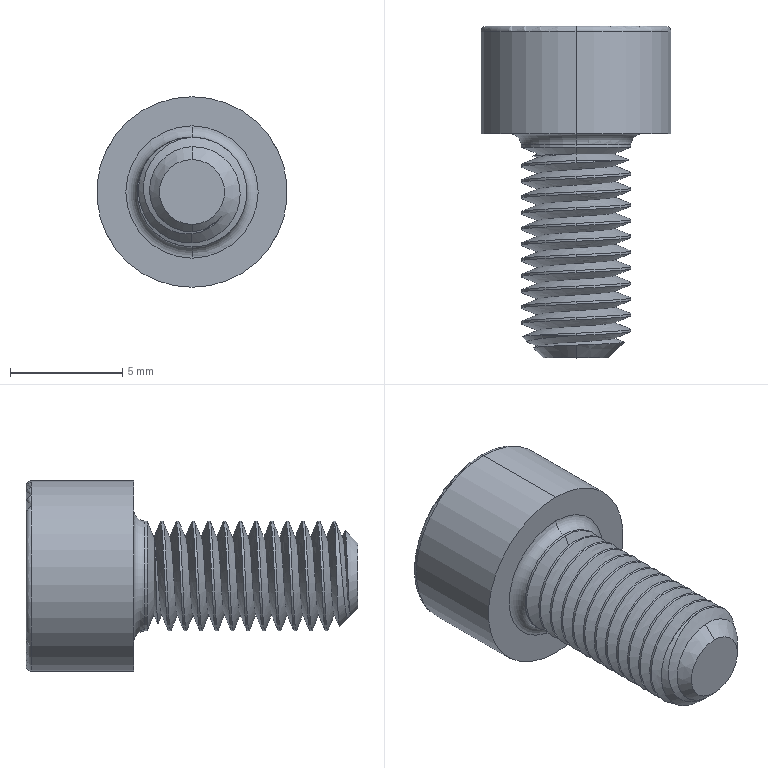Part | STEP file | Parafuso M5 - 10mm | 1 solid | 55 faces | box 8.5 x 14.8 x 8.5 mm | volume 342.133 mm3 | cylinder 28 | plane 10 | cone 9 | torus 6 | spline 2 | commonest cylinder face diameters 4.9 x26 8.5 x2